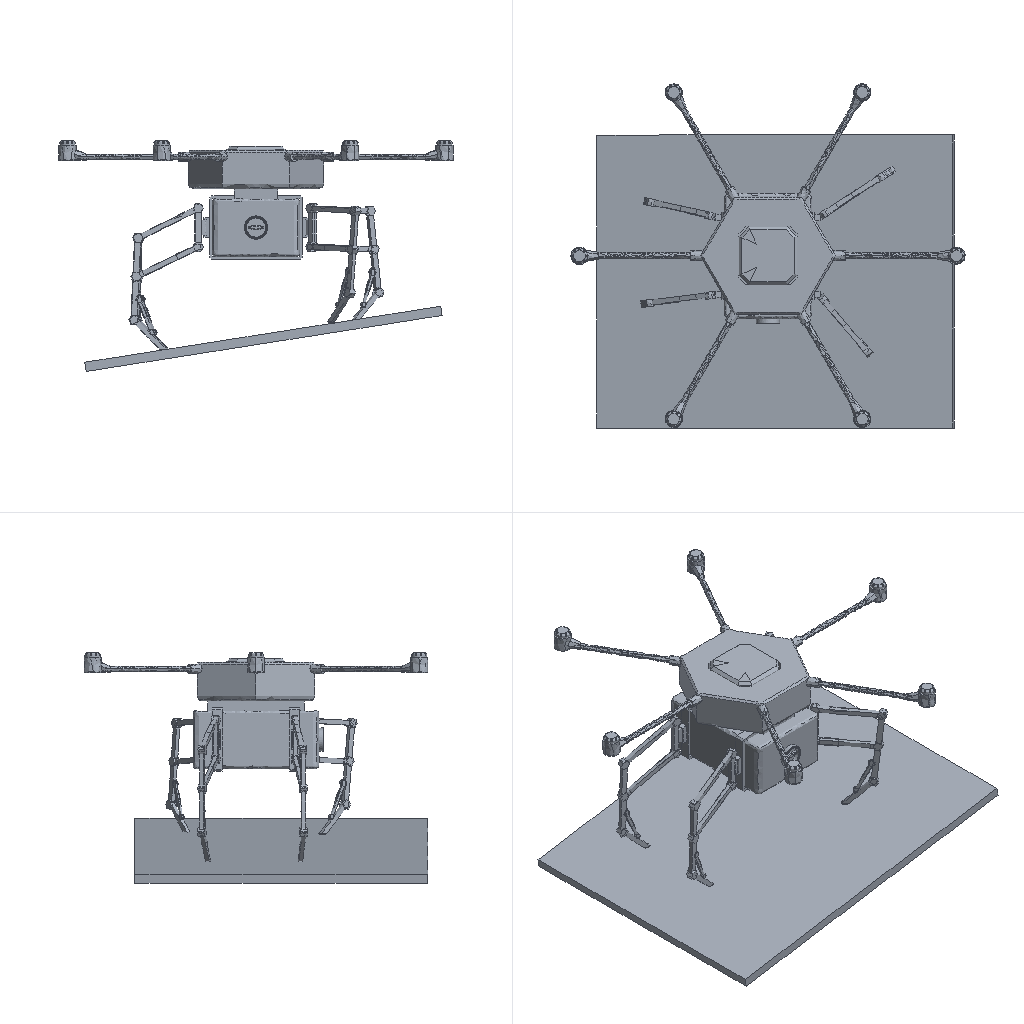Simulation study | ansys workbench
Ansys APDL input file, long lists of numbers shortened:
/batch
/config,noeldb,1     ! force off writing results to database
*get,_wallstrt,active,,time,wall
! ANSYS input file written by Workbench version 2022 R1
! File used for geometry attach:
/title,wbnew--____ (F5)
! ****** Begin Custom Load Command Snippet ******
/COM, ACT Extensions:
/COM,     LSDYNA, 2021.1
/COM,
! ****** End   Custom Load Command Snippet ******
*DIM,_wb_ProjectScratch_dir,string,248
_wb_ProjectScratch_dir(1) = ''
*DIM,_wb_SolverFiles_dir,string,248
_wb_SolverFiles_dir(1) = ''
*DIM,_wb_userfiles_dir,string,248
_wb_userfiles_dir(1) = ''
/com,--- Data in consistent NMM units. See Solving Units in the help system for more information.
/units,MPA
/nopr
/wb,file,start              !  signify a WB generated input file
/prep7
! Turn off shape checking because checks already performed inside WB mesher.
! See help system for more information.
SHPP,OFF,,NOWARN
/nolist
etcon,set             ! allow ANSYS to choose best KEYOP's for 180x elements, resets any applicable keyopt to MAPDL defaults
/com,*********** Nodes for the whole assembly ***********
nblock,3,,112522
(1i9,3e20.9e3)
        1    -5.508865346E+03    -1.475800000E+03    -1.735902488E+03
! (102292 more lines like these left out)
-1
/wb,elem,start            !  set before creation of elements
/com,*********** Elements for Body 1 "xuanyi|dianjizhijia|Chamfer.1" ***********
et,1,187
eblock,19,solid,,480
(19i9)
        1        1        1        1        0        0        0        0       10        0     5151    10218    10222    10326    10253    10413    10440    10416    10414
! (959 more lines like these left out)
-1
/com,*********** Elements for Body 2 "xuanyi|jibi|Pad.1" ***********
et,2,187
eblock,19,solid,,1308
(19i9)
        2        2        2        2        0        0        0        0       10        0    42302    78291    78292    78359    78451    79365    79376    79367    79371
! (2615 more lines like these left out)
-1
/com,*********** Elements for Body 3 "xuanyi|xuanyidianji|CircPattern.1" ***********
et,3,187
eblock,19,solid,,3493
(19i9)
        3        3        3        3        0        0        0        0       10        0     9787    19116    19133    19215    19181    23808    23876    23812    23809
! (6985 more lines like these left out)
-1
/com,*********** Elements for Body 4 "xuanyi|dianjizhijia|Chamfer.1[2]" ***********
et,4,187
eblock,19,solid,,480
(19i9)
        4        4        4        4        0        0        0        0       10        0     4671     9210     9214     9318     9245     9405     9432     9408     9406
! (959 more lines like these left out)
-1
/com,*********** Elements for Body 5 "xuanyi|jibi|Pad.1[2]" ***********
et,5,187
eblock,19,solid,,1308
(19i9)
        5        5        5        5        0        0        0        0       10        0    38378    70386    70387    70454    70546    71460    71471    71462    71466
! (2615 more lines like these left out)
-1
! (50 more sections like these left out)
/wb,elem,end               !  done creating elements
/com,*********** Send User Defined Coordinate System(s) ***********
csys,0
toffst,273.15,  ! Temperature offset from absolute zero
/com,*********** Set Reference Temperature ***********
tref,22.
/wb,mat,start              !  starting to send materials
/com,*********** Send Materials ***********
Temperature = 'TEMP' ! Temperature
MP,DENS,1,7.85e-09,	! tonne mm^-3
MP,ALPX,1,1.2e-05,	! C^-1
MP,C,1,434000000,	! mm^2 s^-2 C^-1
MP,KXX,1,60.5,	! tonne mm s^-3 C^-1
MP,RSVX,1,0.00017,	! ohm mm
MP,EX,1,200000,	! tonne s^-2 mm^-1
MP,NUXY,1,0.3,
MP,MURX,1,10000,
Temperature = 'TEMP' ! Temperature
MP,DENS,2,7.85e-09,	! tonne mm^-3
MP,ALPX,2,1.2e-05,	! C^-1
MP,C,2,434000000,	! mm^2 s^-2 C^-1
MP,KXX,2,60.5,	! tonne mm s^-3 C^-1
MP,RSVX,2,0.00017,	! ohm mm
MP,EX,2,200000,	! tonne s^-2 mm^-1
MP,NUXY,2,0.3,
MP,MURX,2,10000,
Temperature = 'TEMP' ! Temperature
MP,DENS,3,7.85e-09,	! tonne mm^-3
MP,ALPX,3,1.2e-05,	! C^-1
MP,C,3,434000000,	! mm^2 s^-2 C^-1
MP,KXX,3,60.5,	! tonne mm s^-3 C^-1
MP,RSVX,3,0.00017,	! ohm mm
MP,EX,3,200000,	! tonne s^-2 mm^-1
MP,NUXY,3,0.3,
MP,MURX,3,10000,
Temperature = 'TEMP' ! Temperature
MP,DENS,4,7.85e-09,	! tonne mm^-3
MP,ALPX,4,1.2e-05,	! C^-1
MP,C,4,434000000,	! mm^2 s^-2 C^-1
MP,KXX,4,60.5,	! tonne mm s^-3 C^-1
MP,RSVX,4,0.00017,	! ohm mm
MP,EX,4,200000,	! tonne s^-2 mm^-1
MP,NUXY,4,0.3,
MP,MURX,4,10000,
Temperature = 'TEMP' ! Temperature
MP,DENS,5,7.85e-09,	! tonne mm^-3
MP,ALPX,5,1.2e-05,	! C^-1
MP,C,5,434000000,	! mm^2 s^-2 C^-1
MP,KXX,5,60.5,	! tonne mm s^-3 C^-1
MP,RSVX,5,0.00017,	! ohm mm
MP,EX,5,200000,	! tonne s^-2 mm^-1
MP,NUXY,5,0.3,
MP,MURX,5,10000,
Temperature = 'TEMP' ! Temperature
MP,DENS,6,7.85e-09,	! tonne mm^-3
MP,ALPX,6,1.2e-05,	! C^-1
MP,C,6,434000000,	! mm^2 s^-2 C^-1
MP,KXX,6,60.5,	! tonne mm s^-3 C^-1
MP,RSVX,6,0.00017,	! ohm mm
MP,EX,6,200000,	! tonne s^-2 mm^-1
MP,NUXY,6,0.3,
MP,MURX,6,10000,
Temperature = 'TEMP' ! Temperature
MP,DENS,7,7.85e-09,	! tonne mm^-3
MP,ALPX,7,1.2e-05,	! C^-1
MP,C,7,434000000,	! mm^2 s^-2 C^-1
MP,KXX,7,60.5,	! tonne mm s^-3 C^-1
MP,RSVX,7,0.00017,	! ohm mm
MP,EX,7,200000,	! tonne s^-2 mm^-1
MP,NUXY,7,0.3,
MP,MURX,7,10000,
Temperature = 'TEMP' ! Temperature
MP,DENS,8,7.85e-09,	! tonne mm^-3
MP,ALPX,8,1.2e-05,	! C^-1
MP,C,8,434000000,	! mm^2 s^-2 C^-1
MP,KXX,8,60.5,	! tonne mm s^-3 C^-1
MP,RSVX,8,0.00017,	! ohm mm
MP,EX,8,200000,	! tonne s^-2 mm^-1
MP,NUXY,8,0.3,
MP,MURX,8,10000,
Temperature = 'TEMP' ! Temperature
MP,DENS,9,7.85e-09,	! tonne mm^-3
MP,ALPX,9,1.2e-05,	! C^-1
MP,C,9,434000000,	! mm^2 s^-2 C^-1
MP,KXX,9,60.5,	! tonne mm s^-3 C^-1
MP,RSVX,9,0.00017,	! ohm mm
MP,EX,9,200000,	! tonne s^-2 mm^-1
! (416 more lines like these left out)
/wb,mat,end                !  done sending materials
!************************* Model Summary ********************
!xuanyi|dianjizhijia|Chamfer.1,	结构钢,	matid,	1
!xuanyi|jibi|Pad.1,	结构钢,	matid,	2
!xuanyi|xuanyidianji|CircPattern.1,	结构钢,	matid,	3
! (54 more lines like these left out)
*get,_xmin,node,,mnloc,x
*get,_ymin,node,,mnloc,y
*get,_zmin,node,,mnloc,z
*get,_xmax,node,,mxloc,x
*get,_ymax,node,,mxloc,y
*get,_zmax,node,,mxloc,z
_ASMDIAG=(_xmax-_xmin)*(_xmax-_xmin)+(_ymax-_ymin)*(_ymax-_ymin)+(_zmax-_zmin)*(_zmax-_zmin)
_ASMDIAG=SQRT(_ASMDIAG)
/wb,contact,start          !  starting to send contact
/com,*********** Create Contact "接触区域" ***********
/com,            Real Constant Set For Above Contact Is 57 & 56
*set,tid,57
*set,cid,56
r,tid
r,cid
et,tid,170
et,cid,174
eblock,10,,,60
(15i9)
    81076       57       57       57        0    10266    10359    10268    10268    10777    10797    10268    10771
! (59 more lines like these left out)
-1
eblock,10,,,60
(15i9)
    81136       56       56       56        0    10266    10359    10268    10268    10777    10797    10268    10771
! (59 more lines like these left out)
-1
eblock,10,,,74
(15i9)
    81196       56       57       56        0    78221    78228    78223    78223    78711    78720    78223    78709
! (73 more lines like these left out)
-1
eblock,10,,,74
(15i9)
    81270       57       56       57        0    78221    78228    78223    78223    78711    78720    78223    78709
! (73 more lines like these left out)
-1
keyo,cid,8,2               ! auto create asymmetric contact (from Program Controlled setting)
keyo,cid,10,0              ! adjust contact stiffness each NR iteration (from Program Controlled setting)
keyo,cid,12,5              ! bonded always
keyo,cid,18,1              ! small sliding turned on by application
keyo,cid,2,0               ! augmented Lagrange (from Program Controlled setting)
keyo,cid,4,0               ! on Gauss point (from Program Controlled setting)
keyo,cid,9,1               ! ignore initial gaps/penetration
keyo,cid,7,0               ! No Prediction
rmod,tid,3,10.      ! FKN
rmod,tid,5,0.       ! ICONT
rmod,tid,6,0.       ! PINB
rmod,tid,10,0.      ! CNOF
rmod,tid,12,0.      ! FKT
rmod,tid,36,230     ! WB DSID
rmod,cid,3,10.      ! FKN
rmod,cid,5,0.       ! ICONT
rmod,cid,6,0.       ! PINB
rmod,cid,10,0.      ! CNOF
rmod,cid,12,0.      ! FKT
rmod,cid,36,230     ! WB DSID
/com,*********** Create Contact "接触区域 2" ***********
/com,            Real Constant Set For Above Contact Is 59 & 58
*set,tid,59
*set,cid,58
r,tid
r,cid
et,tid,170
et,cid,174
eblock,10,,,78
(15i9)
    81344       59       59       59        0    10248    10250    10360    10360    10635    10655    10360    10640
! (77 more lines like these left out)
-1
eblock,10,,,78
(15i9)
    81422       58       58       58        0    10248    10250    10360    10360    10635    10655    10360    10640
! (77 more lines like these left out)
-1
eblock,10,,,254
(15i9)
    81500       58       59       58        0    18597    18807    18604    18604    20815    20867    18604    20811
! (253 more lines like these left out)
-1
eblock,10,,,254
(15i9)
    81754       59       58       59        0    18597    18807    18604    18604    20815    20867    18604    20811
! (253 more lines like these left out)
-1
keyo,cid,8,2               ! auto create asymmetric contact (from Program Controlled setting)
keyo,cid,10,0              ! adjust contact stiffness each NR iteration (from Program Controlled setting)
keyo,cid,12,5              ! bonded always
keyo,cid,18,1              ! small sliding turned on by application
keyo,cid,2,0               ! augmented Lagrange (from Program Controlled setting)
keyo,cid,4,0               ! on Gauss point (from Program Controlled setting)
keyo,cid,9,1               ! ignore initial gaps/penetration
keyo,cid,7,0               ! No Prediction
rmod,tid,3,10.      ! FKN
rmod,tid,5,0.       ! ICONT
rmod,tid,6,0.       ! PINB
rmod,tid,10,0.      ! CNOF
rmod,tid,12,0.      ! FKT
rmod,tid,36,233     ! WB DSID
rmod,cid,3,10.      ! FKN
rmod,cid,5,0.       ! ICONT
rmod,cid,6,0.       ! PINB
rmod,cid,10,0.      ! CNOF
rmod,cid,12,0.      ! FKT
rmod,cid,36,233     ! WB DSID
/com,*********** Create Contact "接触区域 3" ***********
/com,            Real Constant Set For Above Contact Is 61 & 60
*set,tid,61
*set,cid,60
r,tid
r,cid
et,tid,170
et,cid,174
eblock,10,,,85
(15i9)
    82008       61       61       61        0    78213    78220    78218    78218    78666    78695    78218    78665
! (84 more lines like these left out)
-1
eblock,10,,,85
(15i9)
    82093       60       60       60        0    78213    78220    78218    78218    78666    78695    78218    78665
! (84 more lines like these left out)
-1
eblock,10,,,60
(15i9)
    82178       60       61       60        0    39970    40746    39973    39973    44807    44832    39973    44805
! (59 more lines like these left out)
-1
eblock,10,,,60
(15i9)
    82238       61       60       61        0    39970    40746    39973    39973    44807    44832    39973    44805
! (59 more lines like these left out)
-1
keyo,cid,8,2               ! auto create asymmetric contact (from Program Controlled setting)
keyo,cid,10,0              ! adjust contact stiffness each NR iteration (from Program Controlled setting)
keyo,cid,12,5              ! bonded always
keyo,cid,18,1              ! small sliding turned on by application
keyo,cid,2,0               ! augmented Lagrange (from Program Controlled setting)
keyo,cid,4,0               ! on Gauss point (from Program Controlled setting)
keyo,cid,9,1               ! ignore initial gaps/penetration
keyo,cid,7,0               ! No Prediction
rmod,tid,3,10.      ! FKN
rmod,tid,5,0.       ! ICONT
rmod,tid,6,0.       ! PINB
rmod,tid,10,0.      ! CNOF
rmod,tid,12,0.      ! FKT
rmod,tid,36,236     ! WB DSID
rmod,cid,3,10.      ! FKN
rmod,cid,5,0.       ! ICONT
rmod,cid,6,0.       ! PINB
rmod,cid,10,0.      ! CNOF
rmod,cid,12,0.      ! FKT
rmod,cid,36,236     ! WB DSID
/com,*********** Create Contact "接触区域 8" ***********
/com,            Real Constant Set For Above Contact Is 63 & 62
*set,tid,63
*set,cid,62
r,tid
r,cid
et,tid,170
et,cid,174
eblock,10,,,60
(15i9)
    82298       63       63       63        0     9258     9351     9260     9260     9769     9789     9260     9763
! (59 more lines like these left out)
-1
eblock,10,,,60
(15i9)
    82358       62       62       62        0     9258     9351     9260     9260     9769     9789     9260     9763
! (59 more lines like these left out)
-1
eblock,10,,,74
(15i9)
    82418       62       63       62        0    70316    70323    70318    70318    70806    70815    70318    70804
! (73 more lines like these left out)
-1
eblock,10,,,74
(15i9)
    82492       63       62       63        0    70316    70323    70318    70318    70806    70815    70318    70804
! (73 more lines like these left out)
-1
keyo,cid,8,2               ! auto create asymmetric contact (from Program Controlled setting)
keyo,cid,10,0              ! adjust contact stiffness each NR iteration (from Program Controlled setting)
keyo,cid,12,5              ! bonded always
keyo,cid,18,1              ! small sliding turned on by application
keyo,cid,2,0               ! augmented Lagrange (from Program Controlled setting)
keyo,cid,4,0               ! on Gauss point (from Program Controlled setting)
keyo,cid,9,1               ! ignore initial gaps/penetration
keyo,cid,7,0               ! No Prediction
rmod,tid,3,10.      ! FKN
rmod,tid,5,0.       ! ICONT
rmod,tid,6,0.       ! PINB
rmod,tid,10,0.      ! CNOF
rmod,tid,12,0.      ! FKT
rmod,tid,36,251     ! WB DSID
rmod,cid,3,10.      ! FKN
rmod,cid,5,0.       ! ICONT
rmod,cid,6,0.       ! PINB
rmod,cid,10,0.      ! CNOF
rmod,cid,12,0.      ! FKT
rmod,cid,36,251     ! WB DSID
/com,*********** Create Contact "接触区域 9" ***********
/com,            Real Constant Set For Above Contact Is 65 & 64
*set,tid,65
*set,cid,64
r,tid
r,cid
et,tid,170
et,cid,174
eblock,10,,,78
(15i9)
    82566       65       65       65        0     9240     9242     9352     9352     9627     9647     9352     9632
! (77 more lines like these left out)
-1
eblock,10,,,78
(15i9)
    82644       64       64       64        0     9240     9242     9352     9352     9627     9647     9352     9632
! (77 more lines like these left out)
-1
eblock,10,,,254
(15i9)
    82722       64       65       64        0    12443    12653    12450    12450    14661    14713    12450    14657
! (253 more lines like these left out)
-1
eblock,10,,,254
(15i9)
    82976       65       64       65        0    12443    12653    12450    12450    14661    14713    12450    14657
! (253 more lines like these left out)
-1
keyo,cid,8,2               ! auto create asymmetric contact (from Program Controlled setting)
keyo,cid,10,0              ! adjust contact stiffness each NR iteration (from Program Controlled setting)
keyo,cid,12,5              ! bonded always
keyo,cid,18,1              ! small sliding turned on by application
keyo,cid,2,0               ! augmented Lagrange (from Program Controlled setting)
keyo,cid,4,0               ! on Gauss point (from Program Controlled setting)
keyo,cid,9,1               ! ignore initial gaps/penetration
keyo,cid,7,0               ! No Prediction
rmod,tid,3,10.      ! FKN
rmod,tid,5,0.       ! ICONT
rmod,tid,6,0.       ! PINB
rmod,tid,10,0.      ! CNOF
rmod,tid,12,0.      ! FKT
rmod,tid,36,254     ! WB DSID
rmod,cid,3,10.      ! FKN
rmod,cid,5,0.       ! ICONT
rmod,cid,6,0.       ! PINB
rmod,cid,10,0.      ! CNOF
rmod,cid,12,0.      ! FKT
rmod,cid,36,254     ! WB DSID
! (62 more sections like these left out)
/wb,contact,end            !  done creating contacts
/golist
/wb,load,start             !  starting to send loads
/com,*********** Fixed Supports ***********
CMBLOCK,_FIXEDSU,NODE,     6538
(8i10)
         1         2         3         4         5         6         7         8
! (817 more lines like these left out)
cmsel,s,_FIXEDSU
d,all,all
nsel,all
/com,*********** Define Force Using Surface Effect Elements ***********
local,12,0,0.,0.,0.,0.,0.,0.
csys,0
et,190,154
eblock,10,,,642
(15i9)
    93924      190      190      190       12    40598    40641    40621    40621    48073    48267    40621    48071
! (641 more lines like these left out)
-1
esel,s,type,,190
keyop,190,2,1                ! Apply load in local coordinate system
keyop,190,7,1                ! Use original area so load is constant in large deformation
esel,all
/gst,on,on
fini
*get,_numnode,node,0,count
*get,_numelem,elem,0,count
*get, _MAXELEMNUM, elem, 0, NUM, MAX
*get, _MAXNODENUM, node, 0, NUM, MAX
*get, _MAXELEMTYPE, etyp, 0, NUM, MAX
*get, _MAXREALCONST, real, 0, NUM, MAX
/go
/wb,load,end               !  done creating loads
/com,--- Number of total nodes = %_numnode%
/com,--- Number of contact elements = 13490
/com,--- Number of spring elements = 0
/com,--- Number of bearing elements = 0
/com,--- Number of solid elements = 55575
/com,--- Number of condensed parts = 0
/com,--- Number of total elements = %_numelem%
*get,_wallbsol,active,,time,wall
/com,****************************************************************************
/com,*************************    SOLUTION       ********************************
/com,****************************************************************************
/solu
antype,0                   ! static analysis
_thickRatio=0.164   ! Ratio of thick parts in the model
eqsl,sparse,,,,,1
cntr,print,1               ! print out contact info and also make no initial contact an error
dmpoption,emat,no             ! Don't combine emat file for DANSYS
dmpoption,esav,no             ! Don't combine esav file for DANSYS
nldiag,cont,iter           ! print out contact info each equilibrium iteration
rescontrol,,none                 ! Do not keep any restart files
/com,****************************************************
/com,******************* SOLVE FOR LS 1 OF 1 ****************
esel,s,type,,190
nsle
sfe,all,1,pres,1,0.
sfe,all,2,pres,1,0.
sfe,all,3,pres,1,-2.328
nsel,all
esel,all
/nopr
/gopr
nsub,1,1,1
time,1.
outres,erase
outres,all,none
outres,nsol,all,
outres,rsol,all
outres,eangl,all
outres,etmp,all
outres,veng,all
outres,strs,all,
outres,epel,all,
outres,eppl,all,
outres,cont,all,
! *********** WB SOLVE COMMAND ***********
! check interactive state
*get,ANSINTER_,active,,int
*if,ANSINTER_,ne,0,then
/eof
*endif
solve
/com *************** Write FE CONNECTORS *********
CEWRITE,file,ce,,INTE
/com,****************************************************
/com,*************** FINISHED SOLVE FOR LS 1 *************
*get,_wallasol,active,,time,wall
/nopr
*get,_numnode,node,0,count
*get,_numelem,elem,0,count
*get, _MAXELEMNUM, elem, 0, NUM, MAX
*get, _MAXNODENUM, node, 0, NUM, MAX,,,INTERNAL
*get, _MAXELEMTYPE, etyp, 0, NUM, MAX
*get, _MAXREALCONST, real, 0, NUM, MAX
/gopr
/post1
xmlo,ENCODING,ISO-8859-1
xmlo,parm
/xml,parm,xml
fini
/gopr
*get,_walldone,active,,time,wall
_preptime=(_wallbsol-_wallstrt)*3600
_solvtime=(_wallasol-_wallbsol)*3600
_posttime=(_walldone-_wallasol)*3600
_totaltim=(_walldone-_wallstrt)*3600
*get,_dlbratio,active,0,solu,dlbr
*get,_combtime,active,0,solu,comb
*get,_ssmode,active,0,solu,ssmm
*get,_ndofs,active,0,solu,ndof
*get,_sol_end_time,active,0,set,time
*if,_sol_end_time,eq,1.,then
/fclean				!clean distributed files
*endif
/com,--- Total number of nodes = %_numnode%
/com,--- Total number of elements = %_numelem%
/com,--- Element load balance ratio = %_dlbratio%
/com,--- Time to combine distributed files = %_combtime%
/com,--- Sparse memory mode = %_ssmode%
/com,--- Number of DOF = %_ndofs%
/wb,file,end               ! done with WB generated input